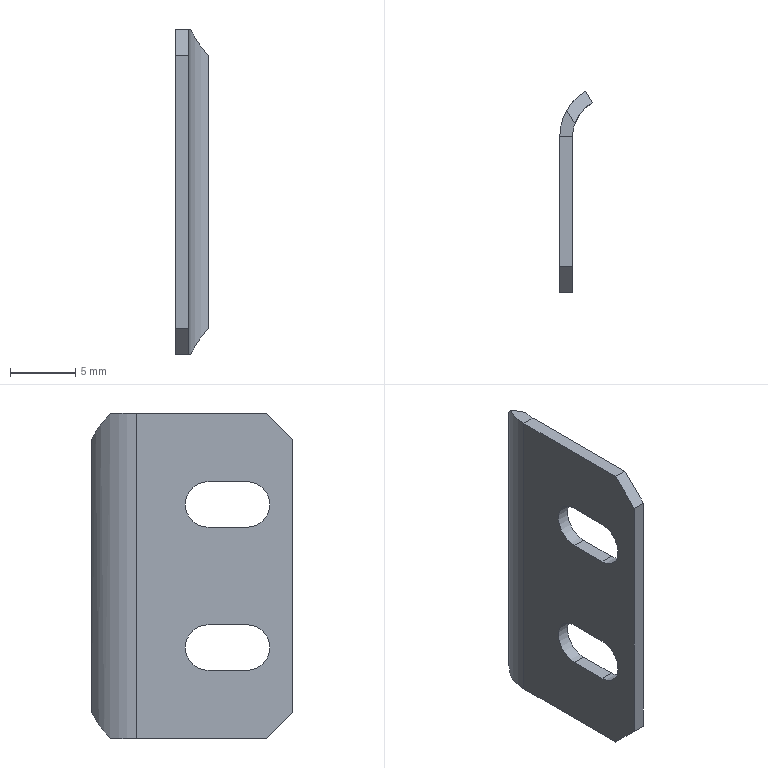Part | SolidWorks | features Chamfer 1, FlatPattern 1, Hem 1, ICE 1, SMBaseFlange 1, SheetMetal 1 | 1 solid | 22 faces | box 2.5 x 15.464 x 25 mm | volume 343.263 mm3 | plane 16 | cylinder 6 | commonest cylinder face diameters 3.5 x4 6 x1 8 x1
STEP:
#1=CARTESIAN_POINT('',(1.,6.5,8.75));
#2=VERTEX_POINT('',#1);
#3=CARTESIAN_POINT('',(1.,3.5,8.75));
#4=VERTEX_POINT('',#3);
#5=CARTESIAN_POINT('',(1.,6.5,8.75));
#6=DIRECTION('',(0.,-1.,0.));
#7=VECTOR('',#6,1000.);
#8=LINE('',#5,#7);
#9=EDGE_CURVE('',#2,#4,#8,.T.);
#10=ORIENTED_EDGE('',*,*,#9,.F.);
#11=CARTESIAN_POINT('',(1.,6.5,5.25));
#12=VERTEX_POINT('',#11);
#13=CARTESIAN_POINT('',(1.,6.5,7.));
#14=DIRECTION('',(1.,0.,0.));
#15=DIRECTION('',(0.,0.,-1.));
#16=AXIS2_PLACEMENT_3D('',#13,#14,#15);
#17=CIRCLE('',#16,1.75);
#18=EDGE_CURVE('',#12,#2,#17,.T.);
#19=ORIENTED_EDGE('',*,*,#18,.F.);
#20=CARTESIAN_POINT('',(1.,3.5,5.25));
#21=VERTEX_POINT('',#20);
#22=CARTESIAN_POINT('',(1.,6.5,5.25));
#23=DIRECTION('',(0.,1.,0.));
#24=VECTOR('',#23,1000.);
#25=LINE('',#22,#24);
#26=EDGE_CURVE('',#21,#12,#25,.T.);
#27=ORIENTED_EDGE('',*,*,#26,.F.);
#28=CARTESIAN_POINT('',(1.,3.5,7.));
#29=DIRECTION('',(1.,0.,0.));
#30=DIRECTION('',(0.,0.,-1.));
#31=AXIS2_PLACEMENT_3D('',#28,#29,#30);
#32=CIRCLE('',#31,1.75);
#33=EDGE_CURVE('',#4,#21,#32,.T.);
#34=ORIENTED_EDGE('',*,*,#33,.F.);
#35=EDGE_LOOP('',(#10,#19,#27,#34));
#36=FACE_BOUND('',#35,.T.);
#37=CARTESIAN_POINT('',(1.,6.5,19.75));
#38=VERTEX_POINT('',#37);
#39=CARTESIAN_POINT('',(1.,3.5,19.75));
#40=VERTEX_POINT('',#39);
#41=CARTESIAN_POINT('',(1.,6.5,19.75));
#42=DIRECTION('',(0.,-1.,0.));
#43=VECTOR('',#42,1000.);
#44=LINE('',#41,#43);
#45=EDGE_CURVE('',#38,#40,#44,.T.);
#46=ORIENTED_EDGE('',*,*,#45,.F.);
#47=CARTESIAN_POINT('',(1.,6.5,16.25));
#48=VERTEX_POINT('',#47);
#49=CARTESIAN_POINT('',(1.,6.5,18.));
#50=DIRECTION('',(1.,0.,0.));
#51=DIRECTION('',(0.,0.,-1.));
#52=AXIS2_PLACEMENT_3D('',#49,#50,#51);
#53=CIRCLE('',#52,1.75);
#54=EDGE_CURVE('',#48,#38,#53,.T.);
#55=ORIENTED_EDGE('',*,*,#54,.F.);
#56=CARTESIAN_POINT('',(1.,3.5,16.25));
#57=VERTEX_POINT('',#56);
#58=CARTESIAN_POINT('',(1.,6.5,16.25));
#59=DIRECTION('',(0.,1.,0.));
#60=VECTOR('',#59,1000.);
#61=LINE('',#58,#60);
#62=EDGE_CURVE('',#57,#48,#61,.T.);
#63=ORIENTED_EDGE('',*,*,#62,.F.);
#64=CARTESIAN_POINT('',(1.,3.5,18.));
#65=DIRECTION('',(1.,0.,0.));
#66=DIRECTION('',(0.,0.,-1.));
#67=AXIS2_PLACEMENT_3D('',#64,#65,#66);
#68=CIRCLE('',#67,1.75);
#69=EDGE_CURVE('',#40,#57,#68,.T.);
#70=ORIENTED_EDGE('',*,*,#69,.F.);
#71=EDGE_LOOP('',(#46,#55,#63,#70));
#72=FACE_BOUND('',#71,.T.);
#73=CARTESIAN_POINT('',(1.,2.,25.));
#74=VERTEX_POINT('',#73);
#75=CARTESIAN_POINT('',(1.,12.,25.));
#76=VERTEX_POINT('',#75);
#77=CARTESIAN_POINT('',(1.,0.,25.));
#78=DIRECTION('',(0.,1.,0.));
#79=VECTOR('',#78,1000.);
#80=LINE('',#77,#79);
#81=EDGE_CURVE('',#74,#76,#80,.T.);
#82=ORIENTED_EDGE('',*,*,#81,.F.);
#83=CARTESIAN_POINT('',(1.,0.,23.));
#84=VERTEX_POINT('',#83);
#85=CARTESIAN_POINT('',(1.,0.,23.));
#86=DIRECTION('',(0.,-0.7071,-0.7071));
#87=VECTOR('',#86,1000.);
#88=LINE('',#85,#87);
#89=EDGE_CURVE('',#74,#84,#88,.T.);
#90=ORIENTED_EDGE('',*,*,#89,.T.);
#91=CARTESIAN_POINT('',(1.,0.,2.));
#92=VERTEX_POINT('',#91);
#93=CARTESIAN_POINT('',(1.,0.,25.));
#94=DIRECTION('',(0.,0.,-1.));
#95=VECTOR('',#94,1000.);
#96=LINE('',#93,#95);
#97=EDGE_CURVE('',#84,#92,#96,.T.);
#98=ORIENTED_EDGE('',*,*,#97,.T.);
#99=CARTESIAN_POINT('',(1.,2.,0.));
#100=VERTEX_POINT('',#99);
#101=CARTESIAN_POINT('',(1.,2.,0.));
#102=DIRECTION('',(0.,0.7071,-0.7071));
#103=VECTOR('',#102,1000.);
#104=LINE('',#101,#103);
#105=EDGE_CURVE('',#92,#100,#104,.T.);
#106=ORIENTED_EDGE('',*,*,#105,.T.);
#107=CARTESIAN_POINT('',(1.,12.,0.));
#108=VERTEX_POINT('',#107);
#109=CARTESIAN_POINT('',(1.,0.,0.));
#110=DIRECTION('',(0.,1.,0.));
#111=VECTOR('',#110,1000.);
#112=LINE('',#109,#111);
#113=EDGE_CURVE('',#100,#108,#112,.T.);
#114=ORIENTED_EDGE('',*,*,#113,.T.);
#115=CARTESIAN_POINT('',(1.,12.,25.));
#116=DIRECTION('',(0.,0.,-1.));
#117=VECTOR('',#116,1000.);
#118=LINE('',#115,#117);
#119=EDGE_CURVE('',#76,#108,#118,.T.);
#120=ORIENTED_EDGE('',*,*,#119,.F.);
#121=EDGE_LOOP('',(#82,#90,#98,#106,#114,#120));
#122=FACE_OUTER_BOUND('',#121,.T.);
#123=CARTESIAN_POINT('',(1.,0.,25.));
#124=DIRECTION('',(-1.,0.,0.));
#125=DIRECTION('',(0.,0.,1.));
#126=AXIS2_PLACEMENT_3D('',#123,#124,#125);
#127=PLANE('',#126);
#128=ADVANCED_FACE('',(#36,#72,#122),#127,.F.);
#129=CARTESIAN_POINT('',(0.,6.5,8.75));
#130=VERTEX_POINT('',#129);
#131=CARTESIAN_POINT('',(0.,6.5,5.25));
#132=VERTEX_POINT('',#131);
#133=CARTESIAN_POINT('',(0.,6.5,7.));
#134=DIRECTION('',(-1.,0.,0.));
#135=DIRECTION('',(0.,0.,1.));
#136=AXIS2_PLACEMENT_3D('',#133,#134,#135);
#137=CIRCLE('',#136,1.75);
#138=EDGE_CURVE('',#130,#132,#137,.T.);
#139=ORIENTED_EDGE('',*,*,#138,.F.);
#140=CARTESIAN_POINT('',(0.,3.5,8.75));
#141=VERTEX_POINT('',#140);
#142=CARTESIAN_POINT('',(0.,0.,8.75));
#143=DIRECTION('',(0.,1.,0.));
#144=VECTOR('',#143,1000.);
#145=LINE('',#142,#144);
#146=EDGE_CURVE('',#141,#130,#145,.T.);
#147=ORIENTED_EDGE('',*,*,#146,.F.);
#148=CARTESIAN_POINT('',(0.,3.5,5.25));
#149=VERTEX_POINT('',#148);
#150=CARTESIAN_POINT('',(0.,3.5,7.));
#151=DIRECTION('',(-1.,0.,0.));
#152=DIRECTION('',(0.,0.,1.));
#153=AXIS2_PLACEMENT_3D('',#150,#151,#152);
#154=CIRCLE('',#153,1.75);
#155=EDGE_CURVE('',#149,#141,#154,.T.);
#156=ORIENTED_EDGE('',*,*,#155,.F.);
#157=CARTESIAN_POINT('',(0.,0.,5.25));
#158=DIRECTION('',(0.,-1.,0.));
#159=VECTOR('',#158,1000.);
#160=LINE('',#157,#159);
#161=EDGE_CURVE('',#132,#149,#160,.T.);
#162=ORIENTED_EDGE('',*,*,#161,.F.);
#163=EDGE_LOOP('',(#139,#147,#156,#162));
#164=FACE_BOUND('',#163,.T.);
#165=CARTESIAN_POINT('',(0.,6.5,19.75));
#166=VERTEX_POINT('',#165);
#167=CARTESIAN_POINT('',(0.,6.5,16.25));
#168=VERTEX_POINT('',#167);
#169=CARTESIAN_POINT('',(0.,6.5,18.));
#170=DIRECTION('',(-1.,0.,0.));
#171=DIRECTION('',(0.,0.,1.));
#172=AXIS2_PLACEMENT_3D('',#169,#170,#171);
#173=CIRCLE('',#172,1.75);
#174=EDGE_CURVE('',#166,#168,#173,.T.);
#175=ORIENTED_EDGE('',*,*,#174,.F.);
#176=CARTESIAN_POINT('',(0.,3.5,19.75));
#177=VERTEX_POINT('',#176);
#178=CARTESIAN_POINT('',(0.,0.,19.75));
#179=DIRECTION('',(0.,1.,0.));
#180=VECTOR('',#179,1000.);
#181=LINE('',#178,#180);
#182=EDGE_CURVE('',#177,#166,#181,.T.);
#183=ORIENTED_EDGE('',*,*,#182,.F.);
#184=CARTESIAN_POINT('',(0.,3.5,16.25));
#185=VERTEX_POINT('',#184);
#186=CARTESIAN_POINT('',(0.,3.5,18.));
#187=DIRECTION('',(-1.,0.,0.));
#188=DIRECTION('',(0.,0.,1.));
#189=AXIS2_PLACEMENT_3D('',#186,#187,#188);
#190=CIRCLE('',#189,1.75);
#191=EDGE_CURVE('',#185,#177,#190,.T.);
#192=ORIENTED_EDGE('',*,*,#191,.F.);
#193=CARTESIAN_POINT('',(0.,0.,16.25));
#194=DIRECTION('',(0.,-1.,0.));
#195=VECTOR('',#194,1000.);
#196=LINE('',#193,#195);
#197=EDGE_CURVE('',#168,#185,#196,.T.);
#198=ORIENTED_EDGE('',*,*,#197,.F.);
#199=EDGE_LOOP('',(#175,#183,#192,#198));
#200=FACE_BOUND('',#199,.T.);
#201=CARTESIAN_POINT('',(0.,0.,23.));
#202=VERTEX_POINT('',#201);
#203=CARTESIAN_POINT('',(0.,0.,2.));
#204=VERTEX_POINT('',#203);
#205=CARTESIAN_POINT('',(0.,0.,25.));
#206=DIRECTION('',(0.,0.,-1.));
#207=VECTOR('',#206,1000.);
#208=LINE('',#205,#207);
#209=EDGE_CURVE('',#202,#204,#208,.T.);
#210=ORIENTED_EDGE('',*,*,#209,.F.);
#211=CARTESIAN_POINT('',(0.,2.,25.));
#212=VERTEX_POINT('',#211);
#213=CARTESIAN_POINT('',(0.,1.,24.));
#214=DIRECTION('',(0.,0.7071,0.7071));
#215=VECTOR('',#214,1000.);
#216=LINE('',#213,#215);
#217=EDGE_CURVE('',#202,#212,#216,.T.);
#218=ORIENTED_EDGE('',*,*,#217,.T.);
#219=CARTESIAN_POINT('',(0.,12.,25.));
#220=VERTEX_POINT('',#219);
#221=CARTESIAN_POINT('',(0.,0.,25.));
#222=DIRECTION('',(0.,1.,0.));
#223=VECTOR('',#222,1000.);
#224=LINE('',#221,#223);
#225=EDGE_CURVE('',#212,#220,#224,.T.);
#226=ORIENTED_EDGE('',*,*,#225,.T.);
#227=CARTESIAN_POINT('',(0.,12.,0.));
#228=VERTEX_POINT('',#227);
#229=CARTESIAN_POINT('',(0.,12.,25.));
#230=DIRECTION('',(0.,0.,-1.));
#231=VECTOR('',#230,1000.);
#232=LINE('',#229,#231);
#233=EDGE_CURVE('',#220,#228,#232,.T.);
#234=ORIENTED_EDGE('',*,*,#233,.T.);
#235=CARTESIAN_POINT('',(0.,2.,0.));
#236=VERTEX_POINT('',#235);
#237=CARTESIAN_POINT('',(0.,0.,0.));
#238=DIRECTION('',(0.,1.,0.));
#239=VECTOR('',#238,1000.);
#240=LINE('',#237,#239);
#241=EDGE_CURVE('',#236,#228,#240,.T.);
#242=ORIENTED_EDGE('',*,*,#241,.F.);
#243=CARTESIAN_POINT('',(0.,-11.5,13.5));
#244=DIRECTION('',(0.,-0.7071,0.7071));
#245=VECTOR('',#244,1000.);
#246=LINE('',#243,#245);
#247=EDGE_CURVE('',#236,#204,#246,.T.);
#248=ORIENTED_EDGE('',*,*,#247,.T.);
#249=EDGE_LOOP('',(#210,#218,#226,#234,#242,#248));
#250=FACE_OUTER_BOUND('',#249,.T.);
#251=CARTESIAN_POINT('',(0.,0.,25.));
#252=DIRECTION('',(-1.,0.,0.));
#253=DIRECTION('',(0.,0.,1.));
#254=AXIS2_PLACEMENT_3D('',#251,#252,#253);
#255=PLANE('',#254);
#256=ADVANCED_FACE('',(#164,#200,#250),#255,.T.);
#257=ORIENTED_EDGE('',*,*,#97,.F.);
#258=CARTESIAN_POINT('',(0.,0.,23.));
#259=DIRECTION('',(-1.,0.,0.));
#260=VECTOR('',#259,1000.);
#261=LINE('',#258,#260);
#262=EDGE_CURVE('',#84,#202,#261,.T.);
#263=ORIENTED_EDGE('',*,*,#262,.T.);
#264=ORIENTED_EDGE('',*,*,#209,.T.);
#265=CARTESIAN_POINT('',(1.,0.,2.));
#266=DIRECTION('',(1.,0.,0.));
#267=VECTOR('',#266,1000.);
#268=LINE('',#265,#267);
#269=EDGE_CURVE('',#204,#92,#268,.T.);
#270=ORIENTED_EDGE('',*,*,#269,.T.);
#271=EDGE_LOOP('',(#257,#263,#264,#270));
#272=FACE_OUTER_BOUND('',#271,.T.);
#273=CARTESIAN_POINT('',(1.,0.,25.));
#274=DIRECTION('',(0.,-1.,0.));
#275=DIRECTION('',(0.,0.,-1.));
#276=AXIS2_PLACEMENT_3D('',#273,#274,#275);
#277=PLANE('',#276);
#278=ADVANCED_FACE('',(#272),#277,.T.);
#279=ORIENTED_EDGE('',*,*,#225,.F.);
#280=CARTESIAN_POINT('',(1.,2.,25.));
#281=DIRECTION('',(1.,0.,0.));
#282=VECTOR('',#281,1000.);
#283=LINE('',#280,#282);
#284=EDGE_CURVE('',#212,#74,#283,.T.);
#285=ORIENTED_EDGE('',*,*,#284,.T.);
#286=ORIENTED_EDGE('',*,*,#81,.T.);
#287=CARTESIAN_POINT('',(1.,12.,25.));
#288=DIRECTION('',(-1.,0.,0.));
#289=VECTOR('',#288,1000.);
#290=LINE('',#287,#289);
#291=EDGE_CURVE('',#76,#220,#290,.T.);
#292=ORIENTED_EDGE('',*,*,#291,.T.);
#293=EDGE_LOOP('',(#279,#285,#286,#292));
#294=FACE_OUTER_BOUND('',#293,.T.);
#295=CARTESIAN_POINT('',(1.,16.,25.));
#296=DIRECTION('',(0.,0.,-1.));
#297=DIRECTION('',(-1.,0.,0.));
#298=AXIS2_PLACEMENT_3D('',#295,#296,#297);
#299=PLANE('',#298);
#300=ADVANCED_FACE('',(#294),#299,.F.);
#301=ORIENTED_EDGE('',*,*,#113,.F.);
#302=CARTESIAN_POINT('',(1.,2.,0.));
#303=DIRECTION('',(-1.,0.,0.));
#304=VECTOR('',#303,1000.);
#305=LINE('',#302,#304);
#306=EDGE_CURVE('',#100,#236,#305,.T.);
#307=ORIENTED_EDGE('',*,*,#306,.T.);
#308=ORIENTED_EDGE('',*,*,#241,.T.);
#309=CARTESIAN_POINT('',(1.,12.,0.));
#310=DIRECTION('',(-1.,0.,0.));
#311=VECTOR('',#310,1000.);
#312=LINE('',#309,#311);
#313=EDGE_CURVE('',#108,#228,#312,.T.);
#314=ORIENTED_EDGE('',*,*,#313,.F.);
#315=EDGE_LOOP('',(#301,#307,#308,#314));
#316=FACE_OUTER_BOUND('',#315,.T.);
#317=CARTESIAN_POINT('',(1.,16.,0.));
#318=DIRECTION('',(0.,0.,-1.));
#319=DIRECTION('',(-1.,0.,0.));
#320=AXIS2_PLACEMENT_3D('',#317,#318,#319);
#321=PLANE('',#320);
#322=ADVANCED_FACE('',(#316),#321,.T.);
#323=CARTESIAN_POINT('',(2.,15.464,2.));
#324=VERTEX_POINT('',#323);
#325=CARTESIAN_POINT('',(2.,15.464,23.));
#326=VERTEX_POINT('',#325);
#327=CARTESIAN_POINT('',(2.,15.464,25.));
#328=DIRECTION('',(0.,0.,1.));
#329=VECTOR('',#328,1000.);
#330=LINE('',#327,#329);
#331=EDGE_CURVE('',#324,#326,#330,.T.);
#332=ORIENTED_EDGE('',*,*,#331,.T.);
#333=CARTESIAN_POINT('',(2.5,14.598,23.));
#334=VERTEX_POINT('',#333);
#335=CARTESIAN_POINT('',(2.5,14.598,23.));
#336=DIRECTION('',(0.5,-0.866,0.));
#337=VECTOR('',#336,1000.);
#338=LINE('',#335,#337);
#339=EDGE_CURVE('',#326,#334,#338,.T.);
#340=ORIENTED_EDGE('',*,*,#339,.T.);
#341=CARTESIAN_POINT('',(2.5,14.598,2.));
#342=VERTEX_POINT('',#341);
#343=CARTESIAN_POINT('',(2.5,14.598,25.));
#344=DIRECTION('',(0.,0.,1.));
#345=VECTOR('',#344,1000.);
#346=LINE('',#343,#345);
#347=EDGE_CURVE('',#342,#334,#346,.T.);
#348=ORIENTED_EDGE('',*,*,#347,.F.);
#349=CARTESIAN_POINT('',(2.5,14.598,2.));
#350=DIRECTION('',(-0.5,0.866,0.));
#351=VECTOR('',#350,1000.);
#352=LINE('',#349,#351);
#353=EDGE_CURVE('',#342,#324,#352,.T.);
#354=ORIENTED_EDGE('',*,*,#353,.T.);
#355=EDGE_LOOP('',(#332,#340,#348,#354));
#356=FACE_OUTER_BOUND('',#355,.T.);
#357=CARTESIAN_POINT('',(2.5,14.598,12.5));
#358=DIRECTION('',(-0.866,-0.5,0.));
#359=DIRECTION('',(0.,0.,1.));
#360=AXIS2_PLACEMENT_3D('',#357,#358,#359);
#361=PLANE('',#360);
#362=ADVANCED_FACE('',(#356),#361,.F.);
#363=CARTESIAN_POINT('',(0.5359,14.,0.));
#364=VERTEX_POINT('',#363);
#365=CARTESIAN_POINT('',(4.,12.,0.));
#366=DIRECTION('',(0.,0.,-1.));
#367=DIRECTION('',(1.,0.,0.));
#368=AXIS2_PLACEMENT_3D('',#365,#366,#367);
#369=CIRCLE('',#368,4.);
#370=EDGE_CURVE('',#228,#364,#369,.T.);
#371=ORIENTED_EDGE('',*,*,#370,.T.);
#372=CARTESIAN_POINT('',(1.15,12.936,0.));
#373=VERTEX_POINT('',#372);
#374=CARTESIAN_POINT('',(2.268,11.,0.));
#375=DIRECTION('',(0.5,-0.866,0.));
#376=VECTOR('',#375,1000.);
#377=LINE('',#374,#376);
#378=EDGE_CURVE('',#364,#373,#377,.T.);
#379=ORIENTED_EDGE('',*,*,#378,.T.);
#380=CARTESIAN_POINT('',(4.,12.,0.));
#381=DIRECTION('',(0.,0.,-1.));
#382=DIRECTION('',(1.,0.,0.));
#383=AXIS2_PLACEMENT_3D('',#380,#381,#382);
#384=CIRCLE('',#383,3.);
#385=EDGE_CURVE('',#108,#373,#384,.T.);
#386=ORIENTED_EDGE('',*,*,#385,.F.);
#387=ORIENTED_EDGE('',*,*,#313,.T.);
#388=EDGE_LOOP('',(#371,#379,#386,#387));
#389=FACE_OUTER_BOUND('',#388,.T.);
#390=CARTESIAN_POINT('',(4.,12.,0.));
#391=DIRECTION('',(0.,0.,-1.));
#392=DIRECTION('',(-1.,0.,0.));
#393=AXIS2_PLACEMENT_3D('',#390,#391,#392);
#394=PLANE('',#393);
#395=ADVANCED_FACE('',(#389),#394,.T.);
#396=CARTESIAN_POINT('',(1.15,12.936,25.));
#397=VERTEX_POINT('',#396);
#398=CARTESIAN_POINT('',(4.,12.,25.));
#399=DIRECTION('',(0.,0.,1.));
#400=DIRECTION('',(1.,0.,0.));
#401=AXIS2_PLACEMENT_3D('',#398,#399,#400);
#402=CIRCLE('',#401,3.);
#403=EDGE_CURVE('',#397,#76,#402,.T.);
#404=ORIENTED_EDGE('',*,*,#403,.F.);
#405=CARTESIAN_POINT('',(0.5359,14.,25.));
#406=VERTEX_POINT('',#405);
#407=CARTESIAN_POINT('',(2.268,11.,25.));
#408=DIRECTION('',(-0.5,0.866,0.));
#409=VECTOR('',#408,1000.);
#410=LINE('',#407,#409);
#411=EDGE_CURVE('',#397,#406,#410,.T.);
#412=ORIENTED_EDGE('',*,*,#411,.T.);
#413=CARTESIAN_POINT('',(4.,12.,25.));
#414=DIRECTION('',(0.,0.,1.));
#415=DIRECTION('',(1.,0.,0.));
#416=AXIS2_PLACEMENT_3D('',#413,#414,#415);
#417=CIRCLE('',#416,4.);
#418=EDGE_CURVE('',#406,#220,#417,.T.);
#419=ORIENTED_EDGE('',*,*,#418,.T.);
#420=ORIENTED_EDGE('',*,*,#291,.F.);
#421=EDGE_LOOP('',(#404,#412,#419,#420));
#422=FACE_OUTER_BOUND('',#421,.T.);
#423=CARTESIAN_POINT('',(4.,12.,25.));
#424=DIRECTION('',(0.,0.,-1.));
#425=DIRECTION('',(-1.,0.,0.));
#426=AXIS2_PLACEMENT_3D('',#423,#424,#425);
#427=PLANE('',#426);
#428=ADVANCED_FACE('',(#422),#427,.F.);
#429=ORIENTED_EDGE('',*,*,#418,.F.);
#430=CARTESIAN_POINT('',(0.5359,14.,25.));
#431=CARTESIAN_POINT('',(0.889,14.612,24.388));
#432=CARTESIAN_POINT('',(1.388,15.111,23.706));
#433=CARTESIAN_POINT('',(2.,15.464,23.));
#434=(BOUNDED_CURVE()B_SPLINE_CURVE(3,(#430,#431,#432,#433),.UNSPECIFIED.,.F.,.F.)B_SPLINE_CURVE_WITH_KNOTS((4,4),(1.047,1.571),.UNSPECIFIED.)CURVE()GEOMETRIC_REPRESENTATION_ITEM()RATIONAL_B_SPLINE_CURVE((1.,0.9773,0.9773,1.))REPRESENTATION_ITEM(''));
#435=EDGE_CURVE('',#406,#326,#434,.T.);
#436=ORIENTED_EDGE('',*,*,#435,.T.);
#437=ORIENTED_EDGE('',*,*,#331,.F.);
#438=CARTESIAN_POINT('',(2.,15.464,2.));
#439=CARTESIAN_POINT('',(1.388,15.111,1.294));
#440=CARTESIAN_POINT('',(0.889,14.612,0.6116));
#441=CARTESIAN_POINT('',(0.5359,14.,0.));
#442=(BOUNDED_CURVE()B_SPLINE_CURVE(3,(#438,#439,#440,#441),.UNSPECIFIED.,.F.,.T.)B_SPLINE_CURVE_WITH_KNOTS((4,4),(1.571,2.094),.UNSPECIFIED.)CURVE()GEOMETRIC_REPRESENTATION_ITEM()RATIONAL_B_SPLINE_CURVE((1.,0.9773,0.9773,1.))REPRESENTATION_ITEM(''));
#443=EDGE_CURVE('',#324,#364,#442,.T.);
#444=ORIENTED_EDGE('',*,*,#443,.T.);
#445=ORIENTED_EDGE('',*,*,#370,.F.);
#446=ORIENTED_EDGE('',*,*,#233,.F.);
#447=EDGE_LOOP('',(#429,#436,#437,#444,#445,#446));
#448=FACE_OUTER_BOUND('',#447,.T.);
#449=CARTESIAN_POINT('',(4.,12.,25.));
#450=DIRECTION('',(0.,0.,1.));
#451=DIRECTION('',(-0.5,0.866,0.));
#452=AXIS2_PLACEMENT_3D('',#449,#450,#451);
#453=CYLINDRICAL_SURFACE('',#452,4.);
#454=ADVANCED_FACE('',(#448),#453,.T.);
#455=ORIENTED_EDGE('',*,*,#347,.T.);
#456=CARTESIAN_POINT('',(2.5,14.598,23.));
#457=CARTESIAN_POINT('',(1.854,14.225,23.746));
#458=CARTESIAN_POINT('',(1.383,13.646,24.444));
#459=CARTESIAN_POINT('',(1.15,12.936,25.));
#460=(BOUNDED_CURVE()B_SPLINE_CURVE(3,(#456,#457,#458,#459),.UNSPECIFIED.,.F.,.T.)B_SPLINE_CURVE_WITH_KNOTS((4,4),(4.712,5.442),.UNSPECIFIED.)CURVE()GEOMETRIC_REPRESENTATION_ITEM()RATIONAL_B_SPLINE_CURVE((1.,0.9561,0.9561,1.))REPRESENTATION_ITEM(''));
#461=EDGE_CURVE('',#334,#397,#460,.T.);
#462=ORIENTED_EDGE('',*,*,#461,.T.);
#463=ORIENTED_EDGE('',*,*,#403,.T.);
#464=ORIENTED_EDGE('',*,*,#119,.T.);
#465=ORIENTED_EDGE('',*,*,#385,.T.);
#466=CARTESIAN_POINT('',(1.15,12.936,0.));
#467=CARTESIAN_POINT('',(1.383,13.646,0.5563));
#468=CARTESIAN_POINT('',(1.854,14.225,1.254));
#469=CARTESIAN_POINT('',(2.5,14.598,2.));
#470=(BOUNDED_CURVE()B_SPLINE_CURVE(3,(#466,#467,#468,#469),.UNSPECIFIED.,.F.,.T.)B_SPLINE_CURVE_WITH_KNOTS((4,4),(3.983,4.712),.UNSPECIFIED.)CURVE()GEOMETRIC_REPRESENTATION_ITEM()RATIONAL_B_SPLINE_CURVE((1.,0.9561,0.9561,1.))REPRESENTATION_ITEM(''));
#471=EDGE_CURVE('',#373,#342,#470,.T.);
#472=ORIENTED_EDGE('',*,*,#471,.T.);
#473=EDGE_LOOP('',(#455,#462,#463,#464,#465,#472));
#474=FACE_OUTER_BOUND('',#473,.T.);
#475=CARTESIAN_POINT('',(4.,12.,25.));
#476=DIRECTION('',(0.,0.,1.));
#477=DIRECTION('',(-0.5,0.866,0.));
#478=AXIS2_PLACEMENT_3D('',#475,#476,#477);
#479=CYLINDRICAL_SURFACE('',#478,3.);
#480=ADVANCED_FACE('',(#474),#479,.F.);
#481=ORIENTED_EDGE('',*,*,#174,.T.);
#482=CARTESIAN_POINT('',(-9.,6.5,16.25));
#483=DIRECTION('',(1.,0.,0.));
#484=VECTOR('',#483,1000.);
#485=LINE('',#482,#484);
#486=EDGE_CURVE('',#168,#48,#485,.T.);
#487=ORIENTED_EDGE('',*,*,#486,.T.);
#488=ORIENTED_EDGE('',*,*,#54,.T.);
#489=CARTESIAN_POINT('',(-9.,6.5,19.75));
#490=DIRECTION('',(1.,0.,0.));
#491=VECTOR('',#490,1000.);
#492=LINE('',#489,#491);
#493=EDGE_CURVE('',#166,#38,#492,.T.);
#494=ORIENTED_EDGE('',*,*,#493,.F.);
#495=EDGE_LOOP('',(#481,#487,#488,#494));
#496=FACE_OUTER_BOUND('',#495,.T.);
#497=CARTESIAN_POINT('',(-9.,6.5,18.));
#498=DIRECTION('',(1.,0.,0.));
#499=DIRECTION('',(0.,0.,-1.));
#500=AXIS2_PLACEMENT_3D('',#497,#498,#499);
#501=CYLINDRICAL_SURFACE('',#500,1.75);
#502=ADVANCED_FACE('',(#496),#501,.F.);
#503=ORIENTED_EDGE('',*,*,#197,.T.);
#504=CARTESIAN_POINT('',(-9.,3.5,16.25));
#505=DIRECTION('',(1.,0.,0.));
#506=VECTOR('',#505,1000.);
#507=LINE('',#504,#506);
#508=EDGE_CURVE('',#185,#57,#507,.T.);
#509=ORIENTED_EDGE('',*,*,#508,.T.);
#510=ORIENTED_EDGE('',*,*,#62,.T.);
#511=ORIENTED_EDGE('',*,*,#486,.F.);
#512=EDGE_LOOP('',(#503,#509,#510,#511));
#513=FACE_OUTER_BOUND('',#512,.T.);
#514=CARTESIAN_POINT('',(-9.,6.5,16.25));
#515=DIRECTION('',(0.,0.,-1.));
#516=DIRECTION('',(-1.,0.,0.));
#517=AXIS2_PLACEMENT_3D('',#514,#515,#516);
#518=PLANE('',#517);
#519=ADVANCED_FACE('',(#513),#518,.F.);
#520=ORIENTED_EDGE('',*,*,#191,.T.);
#521=CARTESIAN_POINT('',(-9.,3.5,19.75));
#522=DIRECTION('',(1.,0.,0.));
#523=VECTOR('',#522,1000.);
#524=LINE('',#521,#523);
#525=EDGE_CURVE('',#177,#40,#524,.T.);
#526=ORIENTED_EDGE('',*,*,#525,.T.);
#527=ORIENTED_EDGE('',*,*,#69,.T.);
#528=ORIENTED_EDGE('',*,*,#508,.F.);
#529=EDGE_LOOP('',(#520,#526,#527,#528));
#530=FACE_OUTER_BOUND('',#529,.T.);
#531=CARTESIAN_POINT('',(-9.,3.5,18.));
#532=DIRECTION('',(1.,0.,0.));
#533=DIRECTION('',(0.,0.,-1.));
#534=AXIS2_PLACEMENT_3D('',#531,#532,#533);
#535=CYLINDRICAL_SURFACE('',#534,1.75);
#536=ADVANCED_FACE('',(#530),#535,.F.);
#537=ORIENTED_EDGE('',*,*,#182,.T.);
#538=ORIENTED_EDGE('',*,*,#493,.T.);
#539=ORIENTED_EDGE('',*,*,#45,.T.);
#540=ORIENTED_EDGE('',*,*,#525,.F.);
#541=EDGE_LOOP('',(#537,#538,#539,#540));
#542=FACE_OUTER_BOUND('',#541,.T.);
#543=CARTESIAN_POINT('',(-9.,6.5,19.75));
#544=DIRECTION('',(0.,0.,1.));
#545=DIRECTION('',(1.,0.,0.));
#546=AXIS2_PLACEMENT_3D('',#543,#544,#545);
#547=PLANE('',#546);
#548=ADVANCED_FACE('',(#542),#547,.F.);
#549=ORIENTED_EDGE('',*,*,#138,.T.);
#550=CARTESIAN_POINT('',(-9.,6.5,5.25));
#551=DIRECTION('',(1.,0.,0.));
#552=VECTOR('',#551,1000.);
#553=LINE('',#550,#552);
#554=EDGE_CURVE('',#132,#12,#553,.T.);
#555=ORIENTED_EDGE('',*,*,#554,.T.);
#556=ORIENTED_EDGE('',*,*,#18,.T.);
#557=CARTESIAN_POINT('',(-9.,6.5,8.75));
#558=DIRECTION('',(1.,0.,0.));
#559=VECTOR('',#558,1000.);
#560=LINE('',#557,#559);
#561=EDGE_CURVE('',#130,#2,#560,.T.);
#562=ORIENTED_EDGE('',*,*,#561,.F.);
#563=EDGE_LOOP('',(#549,#555,#556,#562));
#564=FACE_OUTER_BOUND('',#563,.T.);
#565=CARTESIAN_POINT('',(-9.,6.5,7.));
#566=DIRECTION('',(1.,0.,0.));
#567=DIRECTION('',(0.,0.,-1.));
#568=AXIS2_PLACEMENT_3D('',#565,#566,#567);
#569=CYLINDRICAL_SURFACE('',#568,1.75);
#570=ADVANCED_FACE('',(#564),#569,.F.);
#571=ORIENTED_EDGE('',*,*,#161,.T.);
#572=CARTESIAN_POINT('',(-9.,3.5,5.25));
#573=DIRECTION('',(1.,0.,0.));
#574=VECTOR('',#573,1000.);
#575=LINE('',#572,#574);
#576=EDGE_CURVE('',#149,#21,#575,.T.);
#577=ORIENTED_EDGE('',*,*,#576,.T.);
#578=ORIENTED_EDGE('',*,*,#26,.T.);
#579=ORIENTED_EDGE('',*,*,#554,.F.);
#580=EDGE_LOOP('',(#571,#577,#578,#579));
#581=FACE_OUTER_BOUND('',#580,.T.);
#582=CARTESIAN_POINT('',(-9.,6.5,5.25));
#583=DIRECTION('',(0.,0.,-1.));
#584=DIRECTION('',(0.,1.,0.));
#585=AXIS2_PLACEMENT_3D('',#582,#583,#584);
#586=PLANE('',#585);
#587=ADVANCED_FACE('',(#581),#586,.F.);
#588=ORIENTED_EDGE('',*,*,#155,.T.);
#589=CARTESIAN_POINT('',(-9.,3.5,8.75));
#590=DIRECTION('',(1.,0.,0.));
#591=VECTOR('',#590,1000.);
#592=LINE('',#589,#591);
#593=EDGE_CURVE('',#141,#4,#592,.T.);
#594=ORIENTED_EDGE('',*,*,#593,.T.);
#595=ORIENTED_EDGE('',*,*,#33,.T.);
#596=ORIENTED_EDGE('',*,*,#576,.F.);
#597=EDGE_LOOP('',(#588,#594,#595,#596));
#598=FACE_OUTER_BOUND('',#597,.T.);
#599=CARTESIAN_POINT('',(-9.,3.5,7.));
#600=DIRECTION('',(1.,0.,0.));
#601=DIRECTION('',(0.,0.,-1.));
#602=AXIS2_PLACEMENT_3D('',#599,#600,#601);
#603=CYLINDRICAL_SURFACE('',#602,1.75);
#604=ADVANCED_FACE('',(#598),#603,.F.);
#605=ORIENTED_EDGE('',*,*,#146,.T.);
#606=ORIENTED_EDGE('',*,*,#561,.T.);
#607=ORIENTED_EDGE('',*,*,#9,.T.);
#608=ORIENTED_EDGE('',*,*,#593,.F.);
#609=EDGE_LOOP('',(#605,#606,#607,#608));
#610=FACE_OUTER_BOUND('',#609,.T.);
#611=CARTESIAN_POINT('',(-9.,6.5,8.75));
#612=DIRECTION('',(0.,0.,1.));
#613=DIRECTION('',(1.,0.,0.));
#614=AXIS2_PLACEMENT_3D('',#611,#612,#613);
#615=PLANE('',#614);
#616=ADVANCED_FACE('',(#610),#615,.F.);
#617=ORIENTED_EDGE('',*,*,#461,.F.);
#618=ORIENTED_EDGE('',*,*,#339,.F.);
#619=ORIENTED_EDGE('',*,*,#435,.F.);
#620=ORIENTED_EDGE('',*,*,#411,.F.);
#621=EDGE_LOOP('',(#617,#618,#619,#620));
#622=FACE_OUTER_BOUND('',#621,.T.);
#623=CARTESIAN_POINT('',(2.268,11.,25.));
#624=DIRECTION('',(-0.6124,-0.3536,-0.7071));
#625=DIRECTION('',(-0.5,0.866,0.));
#626=AXIS2_PLACEMENT_3D('',#623,#624,#625);
#627=PLANE('',#626);
#628=ADVANCED_FACE('',(#622),#627,.F.);
#629=ORIENTED_EDGE('',*,*,#471,.F.);
#630=ORIENTED_EDGE('',*,*,#378,.F.);
#631=ORIENTED_EDGE('',*,*,#443,.F.);
#632=ORIENTED_EDGE('',*,*,#353,.F.);
#633=EDGE_LOOP('',(#629,#630,#631,#632));
#634=FACE_OUTER_BOUND('',#633,.T.);
#635=CARTESIAN_POINT('',(2.5,14.598,2.));
#636=DIRECTION('',(0.6124,0.3536,-0.7071));
#637=DIRECTION('',(0.5,-0.866,0.));
#638=AXIS2_PLACEMENT_3D('',#635,#636,#637);
#639=PLANE('',#638);
#640=ADVANCED_FACE('',(#634),#639,.T.);
#641=ORIENTED_EDGE('',*,*,#89,.F.);
#642=ORIENTED_EDGE('',*,*,#284,.F.);
#643=ORIENTED_EDGE('',*,*,#217,.F.);
#644=ORIENTED_EDGE('',*,*,#262,.F.);
#645=EDGE_LOOP('',(#641,#642,#643,#644));
#646=FACE_OUTER_BOUND('',#645,.T.);
#647=CARTESIAN_POINT('',(1.,0.,23.));
#648=DIRECTION('',(0.,-0.7071,0.7071));
#649=DIRECTION('',(1.,0.,0.));
#650=AXIS2_PLACEMENT_3D('',#647,#648,#649);
#651=PLANE('',#650);
#652=ADVANCED_FACE('',(#646),#651,.T.);
#653=ORIENTED_EDGE('',*,*,#105,.F.);
#654=ORIENTED_EDGE('',*,*,#269,.F.);
#655=ORIENTED_EDGE('',*,*,#247,.F.);
#656=ORIENTED_EDGE('',*,*,#306,.F.);
#657=EDGE_LOOP('',(#653,#654,#655,#656));
#658=FACE_OUTER_BOUND('',#657,.T.);
#659=CARTESIAN_POINT('',(1.,2.,0.));
#660=DIRECTION('',(0.,0.7071,0.7071));
#661=DIRECTION('',(-1.,0.,0.));
#662=AXIS2_PLACEMENT_3D('',#659,#660,#661);
#663=PLANE('',#662);
#664=ADVANCED_FACE('',(#658),#663,.F.);
#665=CLOSED_SHELL('',(#128,#256,#278,#300,#322,#362,#395,#428,#454,#480,#502,#519,#536,#548,#570,#587,#604,#616,#628,#640,#652,#664));
#666=MANIFOLD_SOLID_BREP('',#665);
#667=CARTESIAN_POINT('',(0.,0.,0.));
#668=DIRECTION('',(0.,0.,1.));
#669=DIRECTION('',(1.,0.,0.));
#670=AXIS2_PLACEMENT_3D('',#667,#668,#669);
#671=(LENGTH_UNIT()NAMED_UNIT(*)SI_UNIT(.MILLI.,.METRE.));
#672=UNCERTAINTY_MEASURE_WITH_UNIT(LENGTH_MEASURE(0.00001),#671,'','');
#673=(NAMED_UNIT(*)PLANE_ANGLE_UNIT()SI_UNIT($,.RADIAN.));
#674=(NAMED_UNIT(*)SI_UNIT($,.STERADIAN.)SOLID_ANGLE_UNIT());
#675=(GEOMETRIC_REPRESENTATION_CONTEXT(3)GLOBAL_UNCERTAINTY_ASSIGNED_CONTEXT((#672))GLOBAL_UNIT_ASSIGNED_CONTEXT((#671,#673,#674))REPRESENTATION_CONTEXT('',''));
#676=ADVANCED_BREP_SHAPE_REPRESENTATION('',(#666,#670),#675);